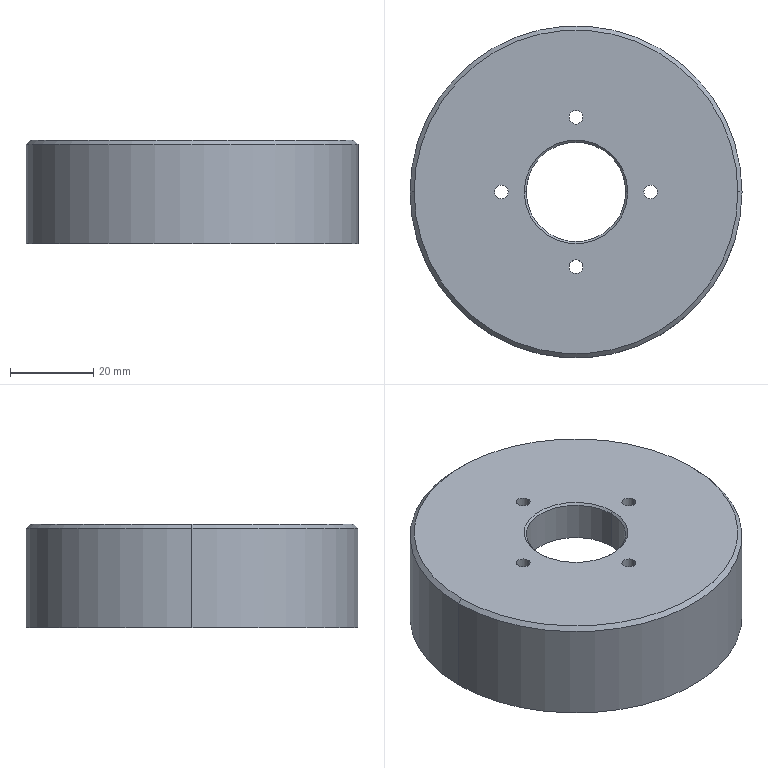Part | SolidWorks | features Chamfer 2, 3DProfileFeature 1, HoleWzd 1, ICE 1, Revolution 1 | 1 solid | 21 faces | box 80 x 80 x 25 mm | volume 62937 mm3 | cylinder 14 | cone 4 | plane 3 | commonest cylinder face diameters 3.3 x8 24 x2 70 x2 80 x2
STEP:
#1=CARTESIAN_POINT('',(-12.,0.,-0.5));
#2=VERTEX_POINT('',#1);
#3=CARTESIAN_POINT('',(12.,0.,-0.5));
#4=VERTEX_POINT('',#3);
#5=CARTESIAN_POINT('',(0.,0.,-0.5));
#6=DIRECTION('',(0.,0.,1.));
#7=DIRECTION('',(-1.,0.,0.));
#8=AXIS2_PLACEMENT_3D('',#5,#6,#7);
#9=CIRCLE('',#8,12.);
#10=EDGE_CURVE('',#2,#4,#9,.T.);
#11=ORIENTED_EDGE('',*,*,#10,.F.);
#12=CARTESIAN_POINT('',(-12.5,0.,0.));
#13=VERTEX_POINT('',#12);
#14=CARTESIAN_POINT('',(-12.,0.,-0.5));
#15=DIRECTION('',(-0.7071,0.,0.7071));
#16=VECTOR('',#15,1000.);
#17=LINE('',#14,#16);
#18=EDGE_CURVE('',#2,#13,#17,.T.);
#19=ORIENTED_EDGE('',*,*,#18,.T.);
#20=CARTESIAN_POINT('',(12.5,0.,0.));
#21=VERTEX_POINT('',#20);
#22=CARTESIAN_POINT('',(0.,0.,0.));
#23=DIRECTION('',(0.,0.,-1.));
#24=DIRECTION('',(-1.,0.,0.));
#25=AXIS2_PLACEMENT_3D('',#22,#23,#24);
#26=CIRCLE('',#25,12.5);
#27=EDGE_CURVE('',#21,#13,#26,.T.);
#28=ORIENTED_EDGE('',*,*,#27,.F.);
#29=CARTESIAN_POINT('',(12.,0.,-0.5));
#30=DIRECTION('',(0.7071,0.,0.7071));
#31=VECTOR('',#30,1000.);
#32=LINE('',#29,#31);
#33=EDGE_CURVE('',#4,#21,#32,.T.);
#34=ORIENTED_EDGE('',*,*,#33,.F.);
#35=EDGE_LOOP('',(#11,#19,#28,#34));
#36=FACE_OUTER_BOUND('',#35,.T.);
#37=CARTESIAN_POINT('',(0.,0.,-0.5));
#38=DIRECTION('',(0.,0.,1.));
#39=DIRECTION('',(1.,0.,0.));
#40=AXIS2_PLACEMENT_3D('',#37,#38,#39);
#41=CONICAL_SURFACE('',#40,12.,0.7854);
#42=ADVANCED_FACE('',(#36),#41,.F.);
#43=CARTESIAN_POINT('',(-1.65,18.,-10.));
#44=VERTEX_POINT('',#43);
#45=CARTESIAN_POINT('',(1.65,18.,-10.));
#46=VERTEX_POINT('',#45);
#47=CARTESIAN_POINT('',(0.,18.,-10.));
#48=DIRECTION('',(0.,0.,1.));
#49=DIRECTION('',(1.,0.,0.));
#50=AXIS2_PLACEMENT_3D('',#47,#48,#49);
#51=CIRCLE('',#50,1.65);
#52=EDGE_CURVE('',#44,#46,#51,.T.);
#53=ORIENTED_EDGE('',*,*,#52,.F.);
#54=CARTESIAN_POINT('',(-1.65,18.,0.));
#55=VERTEX_POINT('',#54);
#56=CARTESIAN_POINT('',(-1.65,18.,0.));
#57=DIRECTION('',(0.,0.,1.));
#58=VECTOR('',#57,1000.);
#59=LINE('',#56,#58);
#60=EDGE_CURVE('',#44,#55,#59,.T.);
#61=ORIENTED_EDGE('',*,*,#60,.T.);
#62=CARTESIAN_POINT('',(1.65,18.,0.));
#63=VERTEX_POINT('',#62);
#64=CARTESIAN_POINT('',(0.,18.,0.));
#65=DIRECTION('',(0.,0.,1.));
#66=DIRECTION('',(1.,0.,0.));
#67=AXIS2_PLACEMENT_3D('',#64,#65,#66);
#68=CIRCLE('',#67,1.65);
#69=EDGE_CURVE('',#55,#63,#68,.T.);
#70=ORIENTED_EDGE('',*,*,#69,.T.);
#71=CARTESIAN_POINT('',(1.65,18.,0.));
#72=DIRECTION('',(0.,0.,1.));
#73=VECTOR('',#72,1000.);
#74=LINE('',#71,#73);
#75=EDGE_CURVE('',#46,#63,#74,.T.);
#76=ORIENTED_EDGE('',*,*,#75,.F.);
#77=EDGE_LOOP('',(#53,#61,#70,#76));
#78=FACE_OUTER_BOUND('',#77,.T.);
#79=CARTESIAN_POINT('',(0.,18.,0.));
#80=DIRECTION('',(0.,0.,1.));
#81=DIRECTION('',(1.,0.,0.));
#82=AXIS2_PLACEMENT_3D('',#79,#80,#81);
#83=CYLINDRICAL_SURFACE('',#82,1.65);
#84=ADVANCED_FACE('',(#78),#83,.F.);
#85=CARTESIAN_POINT('',(-19.65,0.,-10.));
#86=VERTEX_POINT('',#85);
#87=CARTESIAN_POINT('',(-16.35,0.,-10.));
#88=VERTEX_POINT('',#87);
#89=CARTESIAN_POINT('',(-18.,0.,-10.));
#90=DIRECTION('',(0.,0.,1.));
#91=DIRECTION('',(1.,0.,0.));
#92=AXIS2_PLACEMENT_3D('',#89,#90,#91);
#93=CIRCLE('',#92,1.65);
#94=EDGE_CURVE('',#86,#88,#93,.T.);
#95=ORIENTED_EDGE('',*,*,#94,.F.);
#96=CARTESIAN_POINT('',(-19.65,0.,0.));
#97=VERTEX_POINT('',#96);
#98=CARTESIAN_POINT('',(-19.65,0.,0.));
#99=DIRECTION('',(0.,0.,1.));
#100=VECTOR('',#99,1000.);
#101=LINE('',#98,#100);
#102=EDGE_CURVE('',#86,#97,#101,.T.);
#103=ORIENTED_EDGE('',*,*,#102,.T.);
#104=CARTESIAN_POINT('',(-16.35,0.,0.));
#105=VERTEX_POINT('',#104);
#106=CARTESIAN_POINT('',(-18.,0.,0.));
#107=DIRECTION('',(0.,0.,1.));
#108=DIRECTION('',(1.,0.,0.));
#109=AXIS2_PLACEMENT_3D('',#106,#107,#108);
#110=CIRCLE('',#109,1.65);
#111=EDGE_CURVE('',#97,#105,#110,.T.);
#112=ORIENTED_EDGE('',*,*,#111,.T.);
#113=CARTESIAN_POINT('',(-16.35,0.,0.));
#114=DIRECTION('',(0.,0.,1.));
#115=VECTOR('',#114,1000.);
#116=LINE('',#113,#115);
#117=EDGE_CURVE('',#88,#105,#116,.T.);
#118=ORIENTED_EDGE('',*,*,#117,.F.);
#119=EDGE_LOOP('',(#95,#103,#112,#118));
#120=FACE_OUTER_BOUND('',#119,.T.);
#121=CARTESIAN_POINT('',(-18.,0.,0.));
#122=DIRECTION('',(0.,0.,1.));
#123=DIRECTION('',(1.,0.,0.));
#124=AXIS2_PLACEMENT_3D('',#121,#122,#123);
#125=CYLINDRICAL_SURFACE('',#124,1.65);
#126=ADVANCED_FACE('',(#120),#125,.F.);
#127=CARTESIAN_POINT('',(16.35,0.,-10.));
#128=VERTEX_POINT('',#127);
#129=CARTESIAN_POINT('',(19.65,0.,-10.));
#130=VERTEX_POINT('',#129);
#131=CARTESIAN_POINT('',(18.,0.,-10.));
#132=DIRECTION('',(0.,0.,1.));
#133=DIRECTION('',(1.,0.,0.));
#134=AXIS2_PLACEMENT_3D('',#131,#132,#133);
#135=CIRCLE('',#134,1.65);
#136=EDGE_CURVE('',#128,#130,#135,.T.);
#137=ORIENTED_EDGE('',*,*,#136,.F.);
#138=CARTESIAN_POINT('',(16.35,0.,0.));
#139=VERTEX_POINT('',#138);
#140=CARTESIAN_POINT('',(16.35,0.,0.));
#141=DIRECTION('',(0.,0.,1.));
#142=VECTOR('',#141,1000.);
#143=LINE('',#140,#142);
#144=EDGE_CURVE('',#128,#139,#143,.T.);
#145=ORIENTED_EDGE('',*,*,#144,.T.);
#146=CARTESIAN_POINT('',(19.65,0.,0.));
#147=VERTEX_POINT('',#146);
#148=CARTESIAN_POINT('',(18.,0.,0.));
#149=DIRECTION('',(0.,0.,1.));
#150=DIRECTION('',(1.,0.,0.));
#151=AXIS2_PLACEMENT_3D('',#148,#149,#150);
#152=CIRCLE('',#151,1.65);
#153=EDGE_CURVE('',#139,#147,#152,.T.);
#154=ORIENTED_EDGE('',*,*,#153,.T.);
#155=CARTESIAN_POINT('',(19.65,0.,0.));
#156=DIRECTION('',(0.,0.,1.));
#157=VECTOR('',#156,1000.);
#158=LINE('',#155,#157);
#159=EDGE_CURVE('',#130,#147,#158,.T.);
#160=ORIENTED_EDGE('',*,*,#159,.F.);
#161=EDGE_LOOP('',(#137,#145,#154,#160));
#162=FACE_OUTER_BOUND('',#161,.T.);
#163=CARTESIAN_POINT('',(18.,0.,0.));
#164=DIRECTION('',(0.,0.,1.));
#165=DIRECTION('',(1.,0.,0.));
#166=AXIS2_PLACEMENT_3D('',#163,#164,#165);
#167=CYLINDRICAL_SURFACE('',#166,1.65);
#168=ADVANCED_FACE('',(#162),#167,.F.);
#169=CARTESIAN_POINT('',(-1.65,-18.,-10.));
#170=VERTEX_POINT('',#169);
#171=CARTESIAN_POINT('',(1.65,-18.,-10.));
#172=VERTEX_POINT('',#171);
#173=CARTESIAN_POINT('',(0.,-18.,-10.));
#174=DIRECTION('',(0.,0.,1.));
#175=DIRECTION('',(1.,0.,0.));
#176=AXIS2_PLACEMENT_3D('',#173,#174,#175);
#177=CIRCLE('',#176,1.65);
#178=EDGE_CURVE('',#170,#172,#177,.T.);
#179=ORIENTED_EDGE('',*,*,#178,.F.);
#180=CARTESIAN_POINT('',(-1.65,-18.,0.));
#181=VERTEX_POINT('',#180);
#182=CARTESIAN_POINT('',(-1.65,-18.,0.));
#183=DIRECTION('',(0.,0.,1.));
#184=VECTOR('',#183,1000.);
#185=LINE('',#182,#184);
#186=EDGE_CURVE('',#170,#181,#185,.T.);
#187=ORIENTED_EDGE('',*,*,#186,.T.);
#188=CARTESIAN_POINT('',(1.65,-18.,0.));
#189=VERTEX_POINT('',#188);
#190=CARTESIAN_POINT('',(0.,-18.,0.));
#191=DIRECTION('',(0.,0.,1.));
#192=DIRECTION('',(1.,0.,0.));
#193=AXIS2_PLACEMENT_3D('',#190,#191,#192);
#194=CIRCLE('',#193,1.65);
#195=EDGE_CURVE('',#181,#189,#194,.T.);
#196=ORIENTED_EDGE('',*,*,#195,.T.);
#197=CARTESIAN_POINT('',(1.65,-18.,0.));
#198=DIRECTION('',(0.,0.,1.));
#199=VECTOR('',#198,1000.);
#200=LINE('',#197,#199);
#201=EDGE_CURVE('',#172,#189,#200,.T.);
#202=ORIENTED_EDGE('',*,*,#201,.F.);
#203=EDGE_LOOP('',(#179,#187,#196,#202));
#204=FACE_OUTER_BOUND('',#203,.T.);
#205=CARTESIAN_POINT('',(0.,-18.,0.));
#206=DIRECTION('',(0.,0.,1.));
#207=DIRECTION('',(1.,0.,0.));
#208=AXIS2_PLACEMENT_3D('',#205,#206,#207);
#209=CYLINDRICAL_SURFACE('',#208,1.65);
#210=ADVANCED_FACE('',(#204),#209,.F.);
#211=CARTESIAN_POINT('',(-12.,0.,-10.));
#212=VERTEX_POINT('',#211);
#213=CARTESIAN_POINT('',(12.,0.,-10.));
#214=VERTEX_POINT('',#213);
#215=CARTESIAN_POINT('',(0.,0.,-10.));
#216=DIRECTION('',(0.,0.,1.));
#217=DIRECTION('',(1.,0.,0.));
#218=AXIS2_PLACEMENT_3D('',#215,#216,#217);
#219=CIRCLE('',#218,12.);
#220=EDGE_CURVE('',#212,#214,#219,.T.);
#221=ORIENTED_EDGE('',*,*,#220,.F.);
#222=CARTESIAN_POINT('',(-12.,0.,-25.));
#223=DIRECTION('',(0.,0.,1.));
#224=VECTOR('',#223,1000.);
#225=LINE('',#222,#224);
#226=EDGE_CURVE('',#212,#2,#225,.T.);
#227=ORIENTED_EDGE('',*,*,#226,.T.);
#228=ORIENTED_EDGE('',*,*,#10,.T.);
#229=CARTESIAN_POINT('',(12.,0.,-25.));
#230=DIRECTION('',(0.,0.,1.));
#231=VECTOR('',#230,1000.);
#232=LINE('',#229,#231);
#233=EDGE_CURVE('',#214,#4,#232,.T.);
#234=ORIENTED_EDGE('',*,*,#233,.F.);
#235=EDGE_LOOP('',(#221,#227,#228,#234));
#236=FACE_OUTER_BOUND('',#235,.T.);
#237=CARTESIAN_POINT('',(0.,0.,-25.));
#238=DIRECTION('',(0.,0.,1.));
#239=DIRECTION('',(1.,0.,0.));
#240=AXIS2_PLACEMENT_3D('',#237,#238,#239);
#241=CYLINDRICAL_SURFACE('',#240,12.);
#242=ADVANCED_FACE('',(#236),#241,.F.);
#243=CARTESIAN_POINT('',(39.,0.,0.));
#244=VERTEX_POINT('',#243);
#245=CARTESIAN_POINT('',(-39.,0.,0.));
#246=VERTEX_POINT('',#245);
#247=CARTESIAN_POINT('',(0.,0.,0.));
#248=DIRECTION('',(0.,0.,1.));
#249=DIRECTION('',(-1.,0.,0.));
#250=AXIS2_PLACEMENT_3D('',#247,#248,#249);
#251=CIRCLE('',#250,39.);
#252=EDGE_CURVE('',#244,#246,#251,.T.);
#253=ORIENTED_EDGE('',*,*,#252,.F.);
#254=CARTESIAN_POINT('',(40.,0.,-1.));
#255=VERTEX_POINT('',#254);
#256=CARTESIAN_POINT('',(39.,0.,0.));
#257=DIRECTION('',(0.7071,0.,-0.7071));
#258=VECTOR('',#257,1000.);
#259=LINE('',#256,#258);
#260=EDGE_CURVE('',#244,#255,#259,.T.);
#261=ORIENTED_EDGE('',*,*,#260,.T.);
#262=CARTESIAN_POINT('',(-40.,0.,-1.));
#263=VERTEX_POINT('',#262);
#264=CARTESIAN_POINT('',(0.,0.,-1.));
#265=DIRECTION('',(0.,0.,-1.));
#266=DIRECTION('',(-1.,0.,0.));
#267=AXIS2_PLACEMENT_3D('',#264,#265,#266);
#268=CIRCLE('',#267,40.);
#269=EDGE_CURVE('',#263,#255,#268,.T.);
#270=ORIENTED_EDGE('',*,*,#269,.F.);
#271=CARTESIAN_POINT('',(-39.,0.,0.));
#272=DIRECTION('',(-0.7071,0.,-0.7071));
#273=VECTOR('',#272,1000.);
#274=LINE('',#271,#273);
#275=EDGE_CURVE('',#246,#263,#274,.T.);
#276=ORIENTED_EDGE('',*,*,#275,.F.);
#277=EDGE_LOOP('',(#253,#261,#270,#276));
#278=FACE_OUTER_BOUND('',#277,.T.);
#279=CARTESIAN_POINT('',(0.,0.,0.));
#280=DIRECTION('',(0.,0.,-1.));
#281=DIRECTION('',(-1.,0.,0.));
#282=AXIS2_PLACEMENT_3D('',#279,#280,#281);
#283=CONICAL_SURFACE('',#282,39.,0.7854);
#284=ADVANCED_FACE('',(#278),#283,.T.);
#285=CARTESIAN_POINT('',(-35.,0.,-25.));
#286=VERTEX_POINT('',#285);
#287=CARTESIAN_POINT('',(35.,0.,-25.));
#288=VERTEX_POINT('',#287);
#289=CARTESIAN_POINT('',(0.,0.,-25.));
#290=DIRECTION('',(0.,0.,1.));
#291=DIRECTION('',(1.,0.,0.));
#292=AXIS2_PLACEMENT_3D('',#289,#290,#291);
#293=CIRCLE('',#292,35.);
#294=EDGE_CURVE('',#286,#288,#293,.T.);
#295=ORIENTED_EDGE('',*,*,#294,.F.);
#296=CARTESIAN_POINT('',(-35.,0.,-10.));
#297=VERTEX_POINT('',#296);
#298=CARTESIAN_POINT('',(-35.,0.,0.));
#299=DIRECTION('',(0.,0.,1.));
#300=VECTOR('',#299,1000.);
#301=LINE('',#298,#300);
#302=EDGE_CURVE('',#286,#297,#301,.T.);
#303=ORIENTED_EDGE('',*,*,#302,.T.);
#304=CARTESIAN_POINT('',(35.,0.,-10.));
#305=VERTEX_POINT('',#304);
#306=CARTESIAN_POINT('',(0.,0.,-10.));
#307=DIRECTION('',(0.,0.,1.));
#308=DIRECTION('',(1.,0.,0.));
#309=AXIS2_PLACEMENT_3D('',#306,#307,#308);
#310=CIRCLE('',#309,35.);
#311=EDGE_CURVE('',#297,#305,#310,.T.);
#312=ORIENTED_EDGE('',*,*,#311,.T.);
#313=CARTESIAN_POINT('',(35.,0.,0.));
#314=DIRECTION('',(0.,0.,1.));
#315=VECTOR('',#314,1000.);
#316=LINE('',#313,#315);
#317=EDGE_CURVE('',#288,#305,#316,.T.);
#318=ORIENTED_EDGE('',*,*,#317,.F.);
#319=EDGE_LOOP('',(#295,#303,#312,#318));
#320=FACE_OUTER_BOUND('',#319,.T.);
#321=CARTESIAN_POINT('',(0.,0.,0.));
#322=DIRECTION('',(0.,0.,1.));
#323=DIRECTION('',(1.,0.,0.));
#324=AXIS2_PLACEMENT_3D('',#321,#322,#323);
#325=CYLINDRICAL_SURFACE('',#324,35.);
#326=ADVANCED_FACE('',(#320),#325,.F.);
#327=CARTESIAN_POINT('',(40.,0.,-25.));
#328=VERTEX_POINT('',#327);
#329=CARTESIAN_POINT('',(-40.,0.,-25.));
#330=VERTEX_POINT('',#329);
#331=CARTESIAN_POINT('',(0.,0.,-25.));
#332=DIRECTION('',(0.,0.,1.));
#333=DIRECTION('',(1.,0.,0.));
#334=AXIS2_PLACEMENT_3D('',#331,#332,#333);
#335=CIRCLE('',#334,40.);
#336=EDGE_CURVE('',#328,#330,#335,.T.);
#337=ORIENTED_EDGE('',*,*,#336,.T.);
#338=CARTESIAN_POINT('',(-40.,0.,0.));
#339=DIRECTION('',(0.,0.,1.));
#340=VECTOR('',#339,1000.);
#341=LINE('',#338,#340);
#342=EDGE_CURVE('',#330,#263,#341,.T.);
#343=ORIENTED_EDGE('',*,*,#342,.T.);
#344=ORIENTED_EDGE('',*,*,#269,.T.);
#345=CARTESIAN_POINT('',(40.,0.,0.));
#346=DIRECTION('',(0.,0.,1.));
#347=VECTOR('',#346,1000.);
#348=LINE('',#345,#347);
#349=EDGE_CURVE('',#328,#255,#348,.T.);
#350=ORIENTED_EDGE('',*,*,#349,.F.);
#351=EDGE_LOOP('',(#337,#343,#344,#350));
#352=FACE_OUTER_BOUND('',#351,.T.);
#353=CARTESIAN_POINT('',(0.,0.,0.));
#354=DIRECTION('',(0.,0.,1.));
#355=DIRECTION('',(1.,0.,0.));
#356=AXIS2_PLACEMENT_3D('',#353,#354,#355);
#357=CYLINDRICAL_SURFACE('',#356,40.);
#358=ADVANCED_FACE('',(#352),#357,.T.);
#359=ORIENTED_EDGE('',*,*,#27,.T.);
#360=CARTESIAN_POINT('',(0.,0.,0.));
#361=DIRECTION('',(0.,0.,-1.));
#362=DIRECTION('',(-1.,0.,0.));
#363=AXIS2_PLACEMENT_3D('',#360,#361,#362);
#364=CIRCLE('',#363,12.5);
#365=EDGE_CURVE('',#13,#21,#364,.T.);
#366=ORIENTED_EDGE('',*,*,#365,.T.);
#367=EDGE_LOOP('',(#359,#366));
#368=FACE_BOUND('',#367,.T.);
#369=CARTESIAN_POINT('',(0.,18.,0.));
#370=DIRECTION('',(0.,0.,1.));
#371=DIRECTION('',(1.,0.,0.));
#372=AXIS2_PLACEMENT_3D('',#369,#370,#371);
#373=CIRCLE('',#372,1.65);
#374=EDGE_CURVE('',#63,#55,#373,.T.);
#375=ORIENTED_EDGE('',*,*,#374,.F.);
#376=ORIENTED_EDGE('',*,*,#69,.F.);
#377=EDGE_LOOP('',(#375,#376));
#378=FACE_BOUND('',#377,.T.);
#379=CARTESIAN_POINT('',(-18.,0.,0.));
#380=DIRECTION('',(0.,0.,1.));
#381=DIRECTION('',(1.,0.,0.));
#382=AXIS2_PLACEMENT_3D('',#379,#380,#381);
#383=CIRCLE('',#382,1.65);
#384=EDGE_CURVE('',#105,#97,#383,.T.);
#385=ORIENTED_EDGE('',*,*,#384,.F.);
#386=ORIENTED_EDGE('',*,*,#111,.F.);
#387=EDGE_LOOP('',(#385,#386));
#388=FACE_BOUND('',#387,.T.);
#389=CARTESIAN_POINT('',(18.,0.,0.));
#390=DIRECTION('',(0.,0.,1.));
#391=DIRECTION('',(1.,0.,0.));
#392=AXIS2_PLACEMENT_3D('',#389,#390,#391);
#393=CIRCLE('',#392,1.65);
#394=EDGE_CURVE('',#147,#139,#393,.T.);
#395=ORIENTED_EDGE('',*,*,#394,.F.);
#396=ORIENTED_EDGE('',*,*,#153,.F.);
#397=EDGE_LOOP('',(#395,#396));
#398=FACE_BOUND('',#397,.T.);
#399=CARTESIAN_POINT('',(0.,-18.,0.));
#400=DIRECTION('',(0.,0.,1.));
#401=DIRECTION('',(1.,0.,0.));
#402=AXIS2_PLACEMENT_3D('',#399,#400,#401);
#403=CIRCLE('',#402,1.65);
#404=EDGE_CURVE('',#189,#181,#403,.T.);
#405=ORIENTED_EDGE('',*,*,#404,.F.);
#406=ORIENTED_EDGE('',*,*,#195,.F.);
#407=EDGE_LOOP('',(#405,#406));
#408=FACE_BOUND('',#407,.T.);
#409=CARTESIAN_POINT('',(0.,0.,0.));
#410=DIRECTION('',(0.,0.,1.));
#411=DIRECTION('',(-1.,0.,0.));
#412=AXIS2_PLACEMENT_3D('',#409,#410,#411);
#413=CIRCLE('',#412,39.);
#414=EDGE_CURVE('',#246,#244,#413,.T.);
#415=ORIENTED_EDGE('',*,*,#414,.T.);
#416=ORIENTED_EDGE('',*,*,#252,.T.);
#417=EDGE_LOOP('',(#415,#416));
#418=FACE_OUTER_BOUND('',#417,.T.);
#419=CARTESIAN_POINT('',(0.,0.,0.));
#420=DIRECTION('',(0.,0.,-1.));
#421=DIRECTION('',(-1.,0.,0.));
#422=AXIS2_PLACEMENT_3D('',#419,#420,#421);
#423=PLANE('',#422);
#424=ADVANCED_FACE('',(#368,#378,#388,#398,#408,#418),#423,.F.);
#425=ORIENTED_EDGE('',*,*,#342,.F.);
#426=CARTESIAN_POINT('',(0.,0.,-25.));
#427=DIRECTION('',(0.,0.,1.));
#428=DIRECTION('',(1.,0.,0.));
#429=AXIS2_PLACEMENT_3D('',#426,#427,#428);
#430=CIRCLE('',#429,40.);
#431=EDGE_CURVE('',#330,#328,#430,.T.);
#432=ORIENTED_EDGE('',*,*,#431,.T.);
#433=ORIENTED_EDGE('',*,*,#349,.T.);
#434=CARTESIAN_POINT('',(0.,0.,-1.));
#435=DIRECTION('',(0.,0.,-1.));
#436=DIRECTION('',(-1.,0.,0.));
#437=AXIS2_PLACEMENT_3D('',#434,#435,#436);
#438=CIRCLE('',#437,40.);
#439=EDGE_CURVE('',#255,#263,#438,.T.);
#440=ORIENTED_EDGE('',*,*,#439,.T.);
#441=EDGE_LOOP('',(#425,#432,#433,#440));
#442=FACE_OUTER_BOUND('',#441,.T.);
#443=CARTESIAN_POINT('',(0.,0.,0.));
#444=DIRECTION('',(0.,0.,1.));
#445=DIRECTION('',(1.,0.,0.));
#446=AXIS2_PLACEMENT_3D('',#443,#444,#445);
#447=CYLINDRICAL_SURFACE('',#446,40.);
#448=ADVANCED_FACE('',(#442),#447,.T.);
#449=ORIENTED_EDGE('',*,*,#336,.F.);
#450=ORIENTED_EDGE('',*,*,#431,.F.);
#451=EDGE_LOOP('',(#449,#450));
#452=FACE_OUTER_BOUND('',#451,.T.);
#453=CARTESIAN_POINT('',(0.,0.,-25.));
#454=DIRECTION('',(0.,0.,1.));
#455=DIRECTION('',(1.,0.,0.));
#456=AXIS2_PLACEMENT_3D('',#453,#454,#455);
#457=CIRCLE('',#456,35.);
#458=EDGE_CURVE('',#288,#286,#457,.T.);
#459=ORIENTED_EDGE('',*,*,#458,.T.);
#460=ORIENTED_EDGE('',*,*,#294,.T.);
#461=EDGE_LOOP('',(#459,#460));
#462=FACE_BOUND('',#461,.T.);
#463=CARTESIAN_POINT('',(0.,40.,-25.));
#464=DIRECTION('',(0.,0.,1.));
#465=DIRECTION('',(1.,0.,0.));
#466=AXIS2_PLACEMENT_3D('',#463,#464,#465);
#467=PLANE('',#466);
#468=ADVANCED_FACE('',(#452,#462),#467,.F.);
#469=ORIENTED_EDGE('',*,*,#302,.F.);
#470=ORIENTED_EDGE('',*,*,#458,.F.);
#471=ORIENTED_EDGE('',*,*,#317,.T.);
#472=CARTESIAN_POINT('',(0.,0.,-10.));
#473=DIRECTION('',(0.,0.,1.));
#474=DIRECTION('',(1.,0.,0.));
#475=AXIS2_PLACEMENT_3D('',#472,#473,#474);
#476=CIRCLE('',#475,35.);
#477=EDGE_CURVE('',#305,#297,#476,.T.);
#478=ORIENTED_EDGE('',*,*,#477,.T.);
#479=EDGE_LOOP('',(#469,#470,#471,#478));
#480=FACE_OUTER_BOUND('',#479,.T.);
#481=CARTESIAN_POINT('',(0.,0.,0.));
#482=DIRECTION('',(0.,0.,1.));
#483=DIRECTION('',(1.,0.,0.));
#484=AXIS2_PLACEMENT_3D('',#481,#482,#483);
#485=CYLINDRICAL_SURFACE('',#484,35.);
#486=ADVANCED_FACE('',(#480),#485,.F.);
#487=CARTESIAN_POINT('',(0.,18.,-10.));
#488=DIRECTION('',(0.,0.,1.));
#489=DIRECTION('',(1.,0.,0.));
#490=AXIS2_PLACEMENT_3D('',#487,#488,#489);
#491=CIRCLE('',#490,1.65);
#492=EDGE_CURVE('',#46,#44,#491,.T.);
#493=ORIENTED_EDGE('',*,*,#492,.T.);
#494=ORIENTED_EDGE('',*,*,#52,.T.);
#495=EDGE_LOOP('',(#493,#494));
#496=FACE_BOUND('',#495,.T.);
#497=CARTESIAN_POINT('',(-18.,0.,-10.));
#498=DIRECTION('',(0.,0.,1.));
#499=DIRECTION('',(1.,0.,0.));
#500=AXIS2_PLACEMENT_3D('',#497,#498,#499);
#501=CIRCLE('',#500,1.65);
#502=EDGE_CURVE('',#88,#86,#501,.T.);
#503=ORIENTED_EDGE('',*,*,#502,.T.);
#504=ORIENTED_EDGE('',*,*,#94,.T.);
#505=EDGE_LOOP('',(#503,#504));
#506=FACE_BOUND('',#505,.T.);
#507=CARTESIAN_POINT('',(18.,0.,-10.));
#508=DIRECTION('',(0.,0.,1.));
#509=DIRECTION('',(1.,0.,0.));
#510=AXIS2_PLACEMENT_3D('',#507,#508,#509);
#511=CIRCLE('',#510,1.65);
#512=EDGE_CURVE('',#130,#128,#511,.T.);
#513=ORIENTED_EDGE('',*,*,#512,.T.);
#514=ORIENTED_EDGE('',*,*,#136,.T.);
#515=EDGE_LOOP('',(#513,#514));
#516=FACE_BOUND('',#515,.T.);
#517=CARTESIAN_POINT('',(0.,-18.,-10.));
#518=DIRECTION('',(0.,0.,1.));
#519=DIRECTION('',(1.,0.,0.));
#520=AXIS2_PLACEMENT_3D('',#517,#518,#519);
#521=CIRCLE('',#520,1.65);
#522=EDGE_CURVE('',#172,#170,#521,.T.);
#523=ORIENTED_EDGE('',*,*,#522,.T.);
#524=ORIENTED_EDGE('',*,*,#178,.T.);
#525=EDGE_LOOP('',(#523,#524));
#526=FACE_BOUND('',#525,.T.);
#527=CARTESIAN_POINT('',(0.,0.,-10.));
#528=DIRECTION('',(0.,0.,1.));
#529=DIRECTION('',(1.,0.,0.));
#530=AXIS2_PLACEMENT_3D('',#527,#528,#529);
#531=CIRCLE('',#530,12.);
#532=EDGE_CURVE('',#214,#212,#531,.T.);
#533=ORIENTED_EDGE('',*,*,#532,.T.);
#534=ORIENTED_EDGE('',*,*,#220,.T.);
#535=EDGE_LOOP('',(#533,#534));
#536=FACE_BOUND('',#535,.T.);
#537=ORIENTED_EDGE('',*,*,#477,.F.);
#538=ORIENTED_EDGE('',*,*,#311,.F.);
#539=EDGE_LOOP('',(#537,#538));
#540=FACE_OUTER_BOUND('',#539,.T.);
#541=CARTESIAN_POINT('',(0.,35.,-10.));
#542=DIRECTION('',(0.,0.,1.));
#543=DIRECTION('',(1.,0.,0.));
#544=AXIS2_PLACEMENT_3D('',#541,#542,#543);
#545=PLANE('',#544);
#546=ADVANCED_FACE('',(#496,#506,#516,#526,#536,#540),#545,.F.);
#547=ORIENTED_EDGE('',*,*,#260,.F.);
#548=ORIENTED_EDGE('',*,*,#414,.F.);
#549=ORIENTED_EDGE('',*,*,#275,.T.);
#550=ORIENTED_EDGE('',*,*,#439,.F.);
#551=EDGE_LOOP('',(#547,#548,#549,#550));
#552=FACE_OUTER_BOUND('',#551,.T.);
#553=CARTESIAN_POINT('',(0.,0.,0.));
#554=DIRECTION('',(0.,0.,-1.));
#555=DIRECTION('',(-1.,0.,0.));
#556=AXIS2_PLACEMENT_3D('',#553,#554,#555);
#557=CONICAL_SURFACE('',#556,39.,0.7854);
#558=ADVANCED_FACE('',(#552),#557,.T.);
#559=ORIENTED_EDGE('',*,*,#226,.F.);
#560=ORIENTED_EDGE('',*,*,#532,.F.);
#561=ORIENTED_EDGE('',*,*,#233,.T.);
#562=CARTESIAN_POINT('',(0.,0.,-0.5));
#563=DIRECTION('',(0.,0.,1.));
#564=DIRECTION('',(-1.,0.,0.));
#565=AXIS2_PLACEMENT_3D('',#562,#563,#564);
#566=CIRCLE('',#565,12.);
#567=EDGE_CURVE('',#4,#2,#566,.T.);
#568=ORIENTED_EDGE('',*,*,#567,.T.);
#569=EDGE_LOOP('',(#559,#560,#561,#568));
#570=FACE_OUTER_BOUND('',#569,.T.);
#571=CARTESIAN_POINT('',(0.,0.,-25.));
#572=DIRECTION('',(0.,0.,1.));
#573=DIRECTION('',(1.,0.,0.));
#574=AXIS2_PLACEMENT_3D('',#571,#572,#573);
#575=CYLINDRICAL_SURFACE('',#574,12.);
#576=ADVANCED_FACE('',(#570),#575,.F.);
#577=ORIENTED_EDGE('',*,*,#186,.F.);
#578=ORIENTED_EDGE('',*,*,#522,.F.);
#579=ORIENTED_EDGE('',*,*,#201,.T.);
#580=ORIENTED_EDGE('',*,*,#404,.T.);
#581=EDGE_LOOP('',(#577,#578,#579,#580));
#582=FACE_OUTER_BOUND('',#581,.T.);
#583=CARTESIAN_POINT('',(0.,-18.,0.));
#584=DIRECTION('',(0.,0.,1.));
#585=DIRECTION('',(1.,0.,0.));
#586=AXIS2_PLACEMENT_3D('',#583,#584,#585);
#587=CYLINDRICAL_SURFACE('',#586,1.65);
#588=ADVANCED_FACE('',(#582),#587,.F.);
#589=ORIENTED_EDGE('',*,*,#144,.F.);
#590=ORIENTED_EDGE('',*,*,#512,.F.);
#591=ORIENTED_EDGE('',*,*,#159,.T.);
#592=ORIENTED_EDGE('',*,*,#394,.T.);
#593=EDGE_LOOP('',(#589,#590,#591,#592));
#594=FACE_OUTER_BOUND('',#593,.T.);
#595=CARTESIAN_POINT('',(18.,0.,0.));
#596=DIRECTION('',(0.,0.,1.));
#597=DIRECTION('',(1.,0.,0.));
#598=AXIS2_PLACEMENT_3D('',#595,#596,#597);
#599=CYLINDRICAL_SURFACE('',#598,1.65);
#600=ADVANCED_FACE('',(#594),#599,.F.);
#601=ORIENTED_EDGE('',*,*,#102,.F.);
#602=ORIENTED_EDGE('',*,*,#502,.F.);
#603=ORIENTED_EDGE('',*,*,#117,.T.);
#604=ORIENTED_EDGE('',*,*,#384,.T.);
#605=EDGE_LOOP('',(#601,#602,#603,#604));
#606=FACE_OUTER_BOUND('',#605,.T.);
#607=CARTESIAN_POINT('',(-18.,0.,0.));
#608=DIRECTION('',(0.,0.,1.));
#609=DIRECTION('',(1.,0.,0.));
#610=AXIS2_PLACEMENT_3D('',#607,#608,#609);
#611=CYLINDRICAL_SURFACE('',#610,1.65);
#612=ADVANCED_FACE('',(#606),#611,.F.);
#613=ORIENTED_EDGE('',*,*,#60,.F.);
#614=ORIENTED_EDGE('',*,*,#492,.F.);
#615=ORIENTED_EDGE('',*,*,#75,.T.);
#616=ORIENTED_EDGE('',*,*,#374,.T.);
#617=EDGE_LOOP('',(#613,#614,#615,#616));
#618=FACE_OUTER_BOUND('',#617,.T.);
#619=CARTESIAN_POINT('',(0.,18.,0.));
#620=DIRECTION('',(0.,0.,1.));
#621=DIRECTION('',(1.,0.,0.));
#622=AXIS2_PLACEMENT_3D('',#619,#620,#621);
#623=CYLINDRICAL_SURFACE('',#622,1.65);
#624=ADVANCED_FACE('',(#618),#623,.F.);
#625=ORIENTED_EDGE('',*,*,#18,.F.);
#626=ORIENTED_EDGE('',*,*,#567,.F.);
#627=ORIENTED_EDGE('',*,*,#33,.T.);
#628=ORIENTED_EDGE('',*,*,#365,.F.);
#629=EDGE_LOOP('',(#625,#626,#627,#628));
#630=FACE_OUTER_BOUND('',#629,.T.);
#631=CARTESIAN_POINT('',(0.,0.,-0.5));
#632=DIRECTION('',(0.,0.,1.));
#633=DIRECTION('',(1.,0.,0.));
#634=AXIS2_PLACEMENT_3D('',#631,#632,#633);
#635=CONICAL_SURFACE('',#634,12.,0.7854);
#636=ADVANCED_FACE('',(#630),#635,.F.);
#637=CLOSED_SHELL('',(#42,#84,#126,#168,#210,#242,#284,#326,#358,#424,#448,#468,#486,#546,#558,#576,#588,#600,#612,#624,#636));
#638=MANIFOLD_SOLID_BREP('',#637);
#639=CARTESIAN_POINT('',(0.,0.,0.));
#640=DIRECTION('',(0.,0.,1.));
#641=DIRECTION('',(1.,0.,0.));
#642=AXIS2_PLACEMENT_3D('',#639,#640,#641);
#643=(LENGTH_UNIT()NAMED_UNIT(*)SI_UNIT(.MILLI.,.METRE.));
#644=UNCERTAINTY_MEASURE_WITH_UNIT(LENGTH_MEASURE(0.00001),#643,'','');
#645=(NAMED_UNIT(*)PLANE_ANGLE_UNIT()SI_UNIT($,.RADIAN.));
#646=(NAMED_UNIT(*)SI_UNIT($,.STERADIAN.)SOLID_ANGLE_UNIT());
#647=(GEOMETRIC_REPRESENTATION_CONTEXT(3)GLOBAL_UNCERTAINTY_ASSIGNED_CONTEXT((#644))GLOBAL_UNIT_ASSIGNED_CONTEXT((#643,#645,#646))REPRESENTATION_CONTEXT('',''));
#648=ADVANCED_BREP_SHAPE_REPRESENTATION('',(#638,#642),#647);